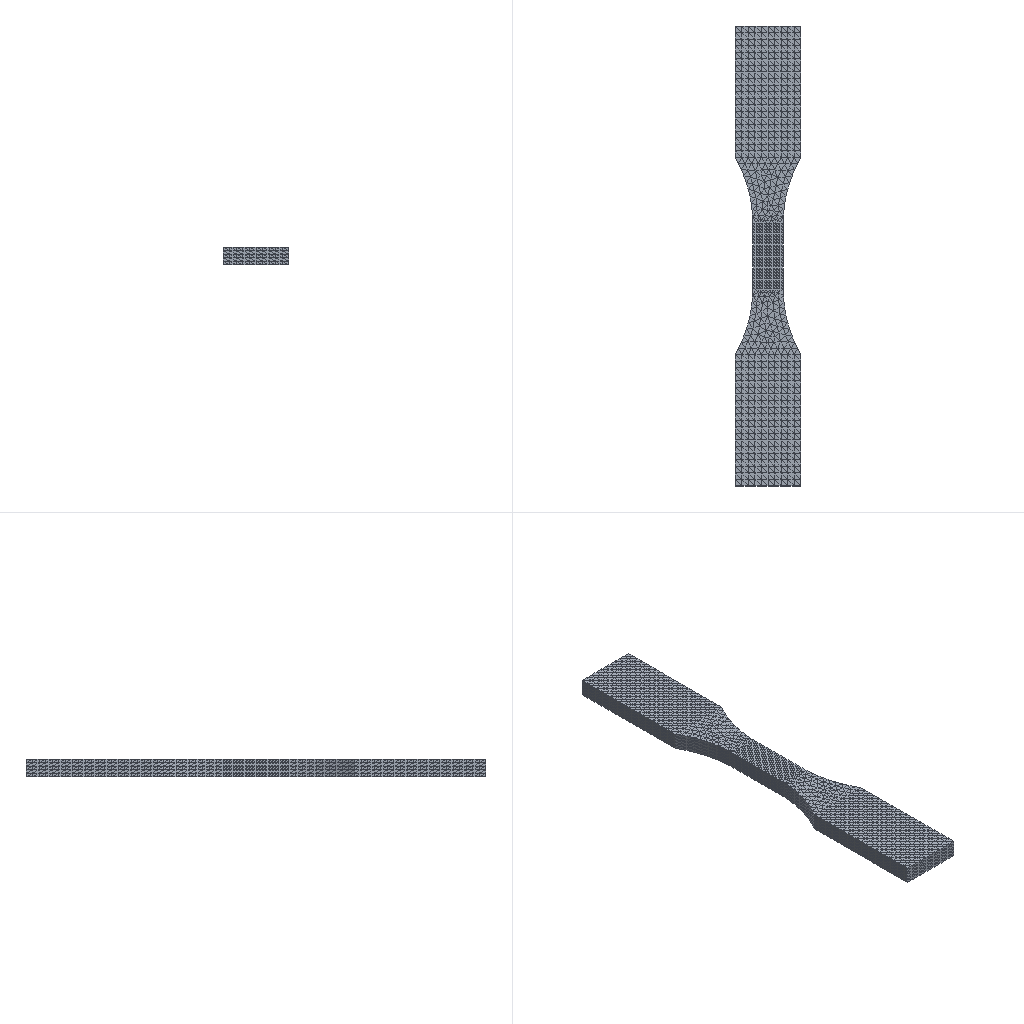Simulation study | abaqus
Set-up summary:
category,name,step,type,value,unit,region
solver,abaqus,,Abaqus/CAE 2024
units,mm-N-s-tonne (MPa),,inferred,E=210000 density=7.85e-09
analysis,Step-1,,dynamic explicit,nlgeom=True; time_period=0.1
mesh,nodes,,,15114
mesh,elements,,,72448
element_type,C3D4,,,72448
material,steel,,E,210000
material,steel,,nu,0.3
material,steel,,density,7.85e-09
material,steel,,yield,753
material,steel,,behaviors,plastic; damage initiation; damage evolution
section,steel,,solid section,,,Set-2
bc,BC-1,Step-1,encastre,[dofs=ENCASTRE],,Set-3
bc,BC-2,Step-1,fixed,"[dofs=rx,ry,rz,x,z n=5]",,Set-4
bc,BC-2,Step-1,displacement,20 [dofs=y],,Set-4
constraint,coupling,,,2
Abaqus input file, long lists of numbers shortened:
*Heading
** Job name: deck Model name: Model-1-Copy
** Generated by: Abaqus/CAE 2024
*Preprint, echo=NO, model=NO, history=NO, contact=NO
**
** PARTS
**
*Part, name=Part-1-new
*Node
      1,          -7.,          15.,           8.
      2,         -15.,          45.,           8.
** (15110 more lines like these left out)
*Element, type=C3D4
   1, 6209, 6210, 6211, 6212
   2, 6209, 6213, 1344, 1336
** (72446 more lines like these left out)
*Nset, nset=Set-1
    4,    7,   64,   65,   66,   67,   68,   69,   70,   71,   72,   73,   74,   75,   76,   77
   78,   79,   80,   81,   82,   83,   84,   85,   86,   87,   88,   89,   90,   91,   92,   93
** (217 more lines like these left out)
*Elset, elset=Set-1
  6369,  6490,  6635,  6741,  6795,  7014,  7052,  7317,  7355,  7394,  7411,  7660,  7694,  8015,  8024,  8027
  8040,  8041,  8049,  8079,  8367,  8504,  8550,  8552,  8630,  8884,  8973,  9062,  9072,  9095,  9177,  9198
** (415 more lines like these left out)
*Nset, nset=Set-2, generate
     1,  15112,      1
*Elset, elset=Set-2, generate
     1,  72448,      1
** Section: Section-1
*Solid Section, elset=Set-2, material=steel
,
*End Part
**
**
** ASSEMBLY
**
*Assembly, name=Assembly
**
*Instance, name=Part-1-new-1, part=Part-1-new
*End Instance
**
*Node
      1,           0.,         106.,           4.
*Node
      2,           0.,        -106.,           4.
*Nset, nset=Set-3
 2,
*Nset, nset=Set-4
 1,
*Nset, nset=m_Set-1
 1,
*Nset, nset=m_Set-2
 2,
*Nset, nset=qw
 1,
*Elset, elset=_s_Surf-1_S3, internal, instance=Part-1-new-1
 68085, 68238, 68254, 68465, 68577, 68610, 68649, 68686, 68713, 68818, 68846, 68922, 69000, 69042, 69069, 69070
 69071, 69072, 69090, 69093, 69166, 69170, 69244, 69267, 69406, 69415, 69649, 69749, 69759, 70021, 70111, 70385
** (3 more lines like these left out)
*Elset, elset=_s_Surf-1_S2, internal, instance=Part-1-new-1
 68606, 71630, 71776
*Elset, elset=_s_Surf-1_S4, internal, instance=Part-1-new-1
 68940, 69086, 69265, 69449, 70424, 70425, 71419, 71533, 71547, 71674, 71876, 71884, 71890, 71925
*Elset, elset=_s_Surf-1_S1, internal, instance=Part-1-new-1
 71021, 71438, 71957
*Surface, type=ELEMENT, name=s_Surf-1
_s_Surf-1_S3, S3
_s_Surf-1_S2, S2
_s_Surf-1_S4, S4
_s_Surf-1_S1, S1
*Elset, elset=_s_Surf-2_S4, internal, instance=Part-1-new-1
 2001, 3996, 4524, 4886, 5753, 5888
*Elset, elset=_s_Surf-2_S3, internal, instance=Part-1-new-1
 2403, 2414, 2572, 2719, 2948, 3035, 3171, 3208, 3210, 3377, 3378, 3581, 3603, 3654, 3671, 3921
 3940, 4041, 4059, 4065, 4142, 4146, 4157, 4269, 4361, 4365, 4372, 4373, 4408, 4419, 4459, 4475
** (4 more lines like these left out)
*Elset, elset=_s_Surf-2_S1, internal, instance=Part-1-new-1
 4374, 4583, 4664, 5852
*Surface, type=ELEMENT, name=s_Surf-2
_s_Surf-2_S4, S4
_s_Surf-2_S3, S3
_s_Surf-2_S1, S1
*Elset, elset=__PickedSurf17_S3, internal, instance=Part-1-new-1
 68085, 68159, 68195, 68238, 68254, 68290, 68401, 68415, 68417, 68419, 68456, 68465, 68469, 68471, 68473, 68478
 68488, 68504, 68507, 68510, 68512, 68516, 68518, 68529, 68536, 68538, 68541, 68543, 68563, 68564, 68577, 68587
** (73 more lines like these left out)
*Elset, elset=__PickedSurf17_S1, internal, instance=Part-1-new-1
 68293, 68396, 68606, 68613, 68984, 69449, 70046, 70159, 70333, 70424, 70713, 71021, 71135, 71160, 71223, 71310
 71321, 71438, 71449, 71516, 71536, 71803, 71884, 71957, 71988, 72070
*Elset, elset=__PickedSurf17_S4, internal, instance=Part-1-new-1
 68068, 68517, 68669, 68940, 69086, 69210, 69265, 69376, 69449, 69896, 70142, 70207, 70292, 70378, 70394, 70414
 70424, 70425, 70464, 70534, 70715, 70841, 70921, 70979, 71264, 71278, 71297, 71342, 71419, 71446, 71481, 71519
** (2 more lines like these left out)
*Elset, elset=__PickedSurf17_S2, internal, instance=Part-1-new-1
 68606, 69265, 69376, 69704, 69750, 70046, 70333, 70748, 71135, 71160, 71223, 71264, 71297, 71373, 71408, 71414
 71434, 71460, 71479, 71630, 71681, 71696, 71776, 71872, 71876, 71915, 71923, 71925, 72010, 72070, 72240, 72411
*Surface, type=ELEMENT, name=_PickedSurf17, internal
__PickedSurf17_S3, S3
__PickedSurf17_S1, S1
__PickedSurf17_S4, S4
__PickedSurf17_S2, S2
*Elset, elset=__PickedSurf18_S3, internal, instance=Part-1-new-1
 1963, 1970, 2001, 2006, 2010, 2015, 2024, 2035, 2055, 2061, 2073, 2074, 2093, 2097, 2119, 2151
 2173, 2179, 2214, 2225, 2255, 2294, 2298, 2304, 2309, 2346, 2350, 2378, 2384, 2394, 2400, 2403
** (74 more lines like these left out)
*Elset, elset=__PickedSurf18_S2, internal, instance=Part-1-new-1
 2020, 2826, 2910, 3136, 3996, 4084, 4107, 4304, 4424, 4474, 5350, 5565, 5606, 5906, 5923, 6184
 6328,
*Elset, elset=__PickedSurf18_S1, internal, instance=Part-1-new-1
 2020, 2310, 2409, 2826, 2981, 3006, 3020, 3222, 3569, 3591, 3682, 3965, 3996, 4189, 4299, 4374
 4424, 4583, 4664, 5565, 5606, 5617, 5852, 5888, 5906, 5907, 5974, 6184, 6328
*Elset, elset=__PickedSurf18_S4, internal, instance=Part-1-new-1
 1949, 1965, 2001, 2464, 3593, 3657, 3861, 3962, 3996, 4015, 4025, 4107, 4126, 4138, 4151, 4154
 4246, 4255, 4333, 4345, 4349, 4524, 4575, 4664, 4666, 4702, 4718, 4748, 4886, 5041, 5093, 5150
** (1 more lines like these left out)
*Surface, type=ELEMENT, name=_PickedSurf18, internal
__PickedSurf18_S3, S3
__PickedSurf18_S2, S2
__PickedSurf18_S4, S4
__PickedSurf18_S1, S1
** Constraint: Constraint-1
*Coupling, constraint name=Constraint-1, ref node=m_Set-1, surface=_PickedSurf17
*Kinematic
** Constraint: Constraint-2
*Coupling, constraint name=Constraint-2, ref node=m_Set-2, surface=_PickedSurf18
*Kinematic
*End Assembly
*Amplitude, name=Amp-1
             0.,              0.,             0.1,              1.
**
** MATERIALS
**
*Material, name=steel
*Damage Initiation, criterion=DUCTILE
 0.29,0.,0.
*Damage Evolution, type=DISPLACEMENT
 0.002,
*Density
 7.85e-09,
*Elastic
210000., 0.3
*Plastic
 753.,   0.
 809., 0.01
 829., 0.02
 842.,  0.1
 895., 0.15
 922.,  0.4
 953.,   1.
1100.,   4.
** ----------------------------------------------------------------
**
** STEP: Step-1
**
*Step, name=Step-1, nlgeom=YES
*Dynamic, Explicit
, 0.1
*Bulk Viscosity
0.06, 1.2
** Mass Scaling: Semi-Automatic
**               Whole Model
*Fixed Mass Scaling, factor=1000.
**
** BOUNDARY CONDITIONS
**
** Name: BC-1 Type: Symmetry/Antisymmetry/Encastre
*Boundary
Set-3, ENCASTRE
** Name: BC-2 Type: Displacement/Rotation
*Boundary, amplitude=Amp-1
Set-4, 1, 1
Set-4, 2, 2, 20.
Set-4, 3, 3
Set-4, 4, 4
Set-4, 5, 5
Set-4, 6, 6
**
** OUTPUT REQUESTS
**
*Restart, write, number interval=1, time marks=NO
**
** FIELD OUTPUT: F-Output-1
**
*Output, field
*Node Output
A, RF, U, V
*Element Output, directions=YES
EVF, LE, PE, PEEQ, PEEQVAVG, S, STATUS
*Contact Output
CSTRESS,
**
** HISTORY OUTPUT: H-Output-1
**
*Output, history
*Energy Output
ALLAE, ALLIE, ALLKE
**
** HISTORY OUTPUT: H-Output-2
**
*Node Output, nset=qw
RF2, U2
*End Step
Results summary:
result,odb.job_status,,,JOB_STATUS_UNKNOWN,"consistent, unstated (Abaqus has no unit system)"
result,steps[0].procedure,Step-1,,"*DYNAMIC, EXPLICIT","consistent, unstated (Abaqus has no unit system)"
result,steps[0].time_period,Step-1,,0.1,"consistent, unstated (Abaqus has no unit system)"
result,steps[0].n_frames,Step-1,,9,"consistent, unstated (Abaqus has no unit system)"
result,steps[0].last_frame.id,Step-1,,171889,"consistent, unstated (Abaqus has no unit system)"
result,steps[0].last_frame.value,Step-1,,0.04,"consistent, unstated (Abaqus has no unit system)"
result,steps[0].last_frame.description,Step-1,,Increment    171889: Step Time =   4.0000E-02,"consistent, unstated (Abaqus has no unit system)"
result,steps[0].completed,Step-1,,False,"consistent, unstated (Abaqus has no unit system)"
result,steps[0].max_U_magnitude,Step-1,,30.477,"consistent, unstated (Abaqus has no unit system)"
result,steps[0].max_S_mises,Step-1,,816.326,"consistent, unstated (Abaqus has no unit system)"
result,steps[0].RF_sum[1],Step-1,,439.915,"consistent, unstated (Abaqus has no unit system)"
result,steps[0].RF_sum[2],Step-1,,-152421,"consistent, unstated (Abaqus has no unit system)"
result,steps[0].RF_sum[3],Step-1,,-3057.31,"consistent, unstated (Abaqus has no unit system)"
result,steps[0].diagnostic.n_increments,Step-1,,16,"consistent, unstated (Abaqus has no unit system)"